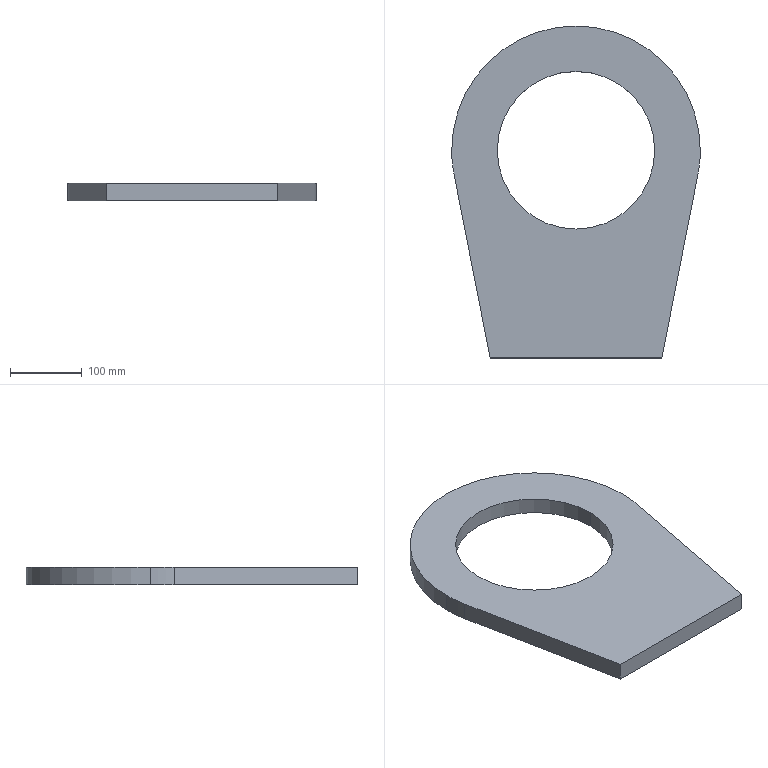Part | SolidWorks | features Extrusion 1, ICE 1 | 1 solid | 13 faces | box 347 x 463.5 x 25 mm | volume 2362679 mm3 | cylinder 7 | plane 6 | commonest cylinder face diameters 347 x3 220 x2 246 x2
STEP:
#1=CARTESIAN_POINT('',(-123.,290.,2.));
#2=VERTEX_POINT('',#1);
#3=CARTESIAN_POINT('',(123.,290.,2.));
#4=VERTEX_POINT('',#3);
#5=CARTESIAN_POINT('',(0.,290.,2.));
#6=DIRECTION('',(0.,0.,1.));
#7=DIRECTION('',(1.,0.,0.));
#8=AXIS2_PLACEMENT_3D('',#5,#6,#7);
#9=CIRCLE('',#8,123.);
#10=EDGE_CURVE('',#2,#4,#9,.T.);
#11=ORIENTED_EDGE('',*,*,#10,.T.);
#12=CARTESIAN_POINT('',(123.,290.,0.));
#13=VERTEX_POINT('',#12);
#14=CARTESIAN_POINT('',(123.,290.,2.));
#15=DIRECTION('',(0.,0.,-1.));
#16=VECTOR('',#15,1000.);
#17=LINE('',#14,#16);
#18=EDGE_CURVE('',#4,#13,#17,.T.);
#19=ORIENTED_EDGE('',*,*,#18,.T.);
#20=CARTESIAN_POINT('',(-123.,290.,0.));
#21=VERTEX_POINT('',#20);
#22=CARTESIAN_POINT('',(0.,290.,0.));
#23=DIRECTION('',(0.,0.,1.));
#24=DIRECTION('',(1.,0.,0.));
#25=AXIS2_PLACEMENT_3D('',#22,#23,#24);
#26=CIRCLE('',#25,123.);
#27=EDGE_CURVE('',#21,#13,#26,.T.);
#28=ORIENTED_EDGE('',*,*,#27,.F.);
#29=CARTESIAN_POINT('',(-123.,290.,2.));
#30=DIRECTION('',(0.,0.,-1.));
#31=VECTOR('',#30,1000.);
#32=LINE('',#29,#31);
#33=EDGE_CURVE('',#2,#21,#32,.T.);
#34=ORIENTED_EDGE('',*,*,#33,.F.);
#35=EDGE_LOOP('',(#11,#19,#28,#34));
#36=FACE_OUTER_BOUND('',#35,.T.);
#37=CARTESIAN_POINT('',(0.,290.,2.));
#38=DIRECTION('',(0.,0.,-1.));
#39=DIRECTION('',(-1.,0.,0.));
#40=AXIS2_PLACEMENT_3D('',#37,#38,#39);
#41=CYLINDRICAL_SURFACE('',#40,123.);
#42=ADVANCED_FACE('',(#36),#41,.F.);
#43=CARTESIAN_POINT('',(-110.,290.,25.));
#44=VERTEX_POINT('',#43);
#45=CARTESIAN_POINT('',(110.,290.,25.));
#46=VERTEX_POINT('',#45);
#47=CARTESIAN_POINT('',(0.,290.,25.));
#48=DIRECTION('',(0.,0.,1.));
#49=DIRECTION('',(1.,0.,0.));
#50=AXIS2_PLACEMENT_3D('',#47,#48,#49);
#51=CIRCLE('',#50,110.);
#52=EDGE_CURVE('',#44,#46,#51,.T.);
#53=ORIENTED_EDGE('',*,*,#52,.T.);
#54=CARTESIAN_POINT('',(110.,290.,2.));
#55=VERTEX_POINT('',#54);
#56=CARTESIAN_POINT('',(110.,290.,25.));
#57=DIRECTION('',(0.,0.,-1.));
#58=VECTOR('',#57,1000.);
#59=LINE('',#56,#58);
#60=EDGE_CURVE('',#46,#55,#59,.T.);
#61=ORIENTED_EDGE('',*,*,#60,.T.);
#62=CARTESIAN_POINT('',(-110.,290.,2.));
#63=VERTEX_POINT('',#62);
#64=CARTESIAN_POINT('',(0.,290.,2.));
#65=DIRECTION('',(0.,0.,1.));
#66=DIRECTION('',(1.,0.,0.));
#67=AXIS2_PLACEMENT_3D('',#64,#65,#66);
#68=CIRCLE('',#67,110.);
#69=EDGE_CURVE('',#63,#55,#68,.T.);
#70=ORIENTED_EDGE('',*,*,#69,.F.);
#71=CARTESIAN_POINT('',(-110.,290.,25.));
#72=DIRECTION('',(0.,0.,-1.));
#73=VECTOR('',#72,1000.);
#74=LINE('',#71,#73);
#75=EDGE_CURVE('',#44,#63,#74,.T.);
#76=ORIENTED_EDGE('',*,*,#75,.F.);
#77=EDGE_LOOP('',(#53,#61,#70,#76));
#78=FACE_OUTER_BOUND('',#77,.T.);
#79=CARTESIAN_POINT('',(0.,290.,25.));
#80=DIRECTION('',(0.,0.,-1.));
#81=DIRECTION('',(-1.,0.,0.));
#82=AXIS2_PLACEMENT_3D('',#79,#80,#81);
#83=CYLINDRICAL_SURFACE('',#82,110.);
#84=ADVANCED_FACE('',(#78),#83,.F.);
#85=CARTESIAN_POINT('',(173.5,290.,25.));
#86=VERTEX_POINT('',#85);
#87=CARTESIAN_POINT('',(-173.5,290.,25.));
#88=VERTEX_POINT('',#87);
#89=CARTESIAN_POINT('',(0.,290.,25.));
#90=DIRECTION('',(0.,0.,1.));
#91=DIRECTION('',(1.,0.,0.));
#92=AXIS2_PLACEMENT_3D('',#89,#90,#91);
#93=CIRCLE('',#92,173.5);
#94=EDGE_CURVE('',#86,#88,#93,.T.);
#95=ORIENTED_EDGE('',*,*,#94,.F.);
#96=CARTESIAN_POINT('',(173.5,290.,0.));
#97=VERTEX_POINT('',#96);
#98=CARTESIAN_POINT('',(173.5,290.,25.));
#99=DIRECTION('',(0.,0.,-1.));
#100=VECTOR('',#99,1000.);
#101=LINE('',#98,#100);
#102=EDGE_CURVE('',#86,#97,#101,.T.);
#103=ORIENTED_EDGE('',*,*,#102,.T.);
#104=CARTESIAN_POINT('',(-173.5,290.,0.));
#105=VERTEX_POINT('',#104);
#106=CARTESIAN_POINT('',(0.,290.,0.));
#107=DIRECTION('',(0.,0.,1.));
#108=DIRECTION('',(1.,0.,0.));
#109=AXIS2_PLACEMENT_3D('',#106,#107,#108);
#110=CIRCLE('',#109,173.5);
#111=EDGE_CURVE('',#97,#105,#110,.T.);
#112=ORIENTED_EDGE('',*,*,#111,.T.);
#113=CARTESIAN_POINT('',(-173.5,290.,25.));
#114=DIRECTION('',(0.,0.,-1.));
#115=VECTOR('',#114,1000.);
#116=LINE('',#113,#115);
#117=EDGE_CURVE('',#88,#105,#116,.T.);
#118=ORIENTED_EDGE('',*,*,#117,.F.);
#119=EDGE_LOOP('',(#95,#103,#112,#118));
#120=FACE_OUTER_BOUND('',#119,.T.);
#121=CARTESIAN_POINT('',(0.,290.,25.));
#122=DIRECTION('',(0.,0.,-1.));
#123=DIRECTION('',(-1.,0.,0.));
#124=AXIS2_PLACEMENT_3D('',#121,#122,#123);
#125=CYLINDRICAL_SURFACE('',#124,173.5);
#126=ADVANCED_FACE('',(#120),#125,.T.);
#127=CARTESIAN_POINT('',(-170.265,256.654,25.));
#128=VERTEX_POINT('',#127);
#129=CARTESIAN_POINT('',(0.,290.,25.));
#130=DIRECTION('',(0.,0.,1.));
#131=DIRECTION('',(1.,0.,0.));
#132=AXIS2_PLACEMENT_3D('',#129,#130,#131);
#133=CIRCLE('',#132,173.5);
#134=EDGE_CURVE('',#88,#128,#133,.T.);
#135=ORIENTED_EDGE('',*,*,#134,.F.);
#136=ORIENTED_EDGE('',*,*,#117,.T.);
#137=CARTESIAN_POINT('',(-170.265,256.654,0.));
#138=VERTEX_POINT('',#137);
#139=CARTESIAN_POINT('',(0.,290.,0.));
#140=DIRECTION('',(0.,0.,1.));
#141=DIRECTION('',(1.,0.,0.));
#142=AXIS2_PLACEMENT_3D('',#139,#140,#141);
#143=CIRCLE('',#142,173.5);
#144=EDGE_CURVE('',#105,#138,#143,.T.);
#145=ORIENTED_EDGE('',*,*,#144,.T.);
#146=CARTESIAN_POINT('',(-170.265,256.654,25.));
#147=DIRECTION('',(0.,0.,-1.));
#148=VECTOR('',#147,1000.);
#149=LINE('',#146,#148);
#150=EDGE_CURVE('',#128,#138,#149,.T.);
#151=ORIENTED_EDGE('',*,*,#150,.F.);
#152=EDGE_LOOP('',(#135,#136,#145,#151));
#153=FACE_OUTER_BOUND('',#152,.T.);
#154=CARTESIAN_POINT('',(0.,290.,25.));
#155=DIRECTION('',(0.,0.,-1.));
#156=DIRECTION('',(-1.,0.,0.));
#157=AXIS2_PLACEMENT_3D('',#154,#155,#156);
#158=CYLINDRICAL_SURFACE('',#157,173.5);
#159=ADVANCED_FACE('',(#153),#158,.T.);
#160=CARTESIAN_POINT('',(-120.,0.,0.));
#161=VERTEX_POINT('',#160);
#162=CARTESIAN_POINT('',(-120.,0.,0.));
#163=DIRECTION('',(0.1922,-0.9814,0.));
#164=VECTOR('',#163,1000.);
#165=LINE('',#162,#164);
#166=EDGE_CURVE('',#138,#161,#165,.T.);
#167=ORIENTED_EDGE('',*,*,#166,.F.);
#168=ORIENTED_EDGE('',*,*,#144,.F.);
#169=ORIENTED_EDGE('',*,*,#111,.F.);
#170=CARTESIAN_POINT('',(170.265,256.654,0.));
#171=VERTEX_POINT('',#170);
#172=CARTESIAN_POINT('',(0.,290.,0.));
#173=DIRECTION('',(0.,0.,1.));
#174=DIRECTION('',(1.,0.,0.));
#175=AXIS2_PLACEMENT_3D('',#172,#173,#174);
#176=CIRCLE('',#175,173.5);
#177=EDGE_CURVE('',#171,#97,#176,.T.);
#178=ORIENTED_EDGE('',*,*,#177,.F.);
#179=CARTESIAN_POINT('',(120.,0.,0.));
#180=VERTEX_POINT('',#179);
#181=CARTESIAN_POINT('',(120.,0.,0.));
#182=DIRECTION('',(0.1922,0.9814,0.));
#183=VECTOR('',#182,1000.);
#184=LINE('',#181,#183);
#185=EDGE_CURVE('',#180,#171,#184,.T.);
#186=ORIENTED_EDGE('',*,*,#185,.F.);
#187=CARTESIAN_POINT('',(-120.,0.,0.));
#188=DIRECTION('',(1.,0.,0.));
#189=VECTOR('',#188,1000.);
#190=LINE('',#187,#189);
#191=EDGE_CURVE('',#161,#180,#190,.T.);
#192=ORIENTED_EDGE('',*,*,#191,.F.);
#193=EDGE_LOOP('',(#167,#168,#169,#178,#186,#192));
#194=FACE_OUTER_BOUND('',#193,.T.);
#195=ORIENTED_EDGE('',*,*,#27,.T.);
#196=CARTESIAN_POINT('',(0.,290.,0.));
#197=DIRECTION('',(0.,0.,1.));
#198=DIRECTION('',(1.,0.,0.));
#199=AXIS2_PLACEMENT_3D('',#196,#197,#198);
#200=CIRCLE('',#199,123.);
#201=EDGE_CURVE('',#13,#21,#200,.T.);
#202=ORIENTED_EDGE('',*,*,#201,.T.);
#203=EDGE_LOOP('',(#195,#202));
#204=FACE_BOUND('',#203,.T.);
#205=CARTESIAN_POINT('',(0.,290.,0.));
#206=DIRECTION('',(0.,0.,1.));
#207=DIRECTION('',(1.,0.,0.));
#208=AXIS2_PLACEMENT_3D('',#205,#206,#207);
#209=PLANE('',#208);
#210=ADVANCED_FACE('',(#194,#204),#209,.F.);
#211=CARTESIAN_POINT('',(-120.,0.,25.));
#212=VERTEX_POINT('',#211);
#213=CARTESIAN_POINT('',(-120.,0.,25.));
#214=DIRECTION('',(0.1922,-0.9814,0.));
#215=VECTOR('',#214,1000.);
#216=LINE('',#213,#215);
#217=EDGE_CURVE('',#128,#212,#216,.T.);
#218=ORIENTED_EDGE('',*,*,#217,.T.);
#219=CARTESIAN_POINT('',(120.,0.,25.));
#220=VERTEX_POINT('',#219);
#221=CARTESIAN_POINT('',(-120.,0.,25.));
#222=DIRECTION('',(1.,0.,0.));
#223=VECTOR('',#222,1000.);
#224=LINE('',#221,#223);
#225=EDGE_CURVE('',#212,#220,#224,.T.);
#226=ORIENTED_EDGE('',*,*,#225,.T.);
#227=CARTESIAN_POINT('',(170.265,256.654,25.));
#228=VERTEX_POINT('',#227);
#229=CARTESIAN_POINT('',(120.,0.,25.));
#230=DIRECTION('',(0.1922,0.9814,0.));
#231=VECTOR('',#230,1000.);
#232=LINE('',#229,#231);
#233=EDGE_CURVE('',#220,#228,#232,.T.);
#234=ORIENTED_EDGE('',*,*,#233,.T.);
#235=CARTESIAN_POINT('',(0.,290.,25.));
#236=DIRECTION('',(0.,0.,1.));
#237=DIRECTION('',(1.,0.,0.));
#238=AXIS2_PLACEMENT_3D('',#235,#236,#237);
#239=CIRCLE('',#238,173.5);
#240=EDGE_CURVE('',#228,#86,#239,.T.);
#241=ORIENTED_EDGE('',*,*,#240,.T.);
#242=ORIENTED_EDGE('',*,*,#94,.T.);
#243=ORIENTED_EDGE('',*,*,#134,.T.);
#244=EDGE_LOOP('',(#218,#226,#234,#241,#242,#243));
#245=FACE_OUTER_BOUND('',#244,.T.);
#246=ORIENTED_EDGE('',*,*,#52,.F.);
#247=CARTESIAN_POINT('',(0.,290.,25.));
#248=DIRECTION('',(0.,0.,1.));
#249=DIRECTION('',(1.,0.,0.));
#250=AXIS2_PLACEMENT_3D('',#247,#248,#249);
#251=CIRCLE('',#250,110.);
#252=EDGE_CURVE('',#46,#44,#251,.T.);
#253=ORIENTED_EDGE('',*,*,#252,.F.);
#254=EDGE_LOOP('',(#246,#253));
#255=FACE_BOUND('',#254,.T.);
#256=CARTESIAN_POINT('',(0.,290.,25.));
#257=DIRECTION('',(0.,0.,1.));
#258=DIRECTION('',(1.,0.,0.));
#259=AXIS2_PLACEMENT_3D('',#256,#257,#258);
#260=PLANE('',#259);
#261=ADVANCED_FACE('',(#245,#255),#260,.T.);
#262=ORIENTED_EDGE('',*,*,#166,.T.);
#263=CARTESIAN_POINT('',(-120.,0.,25.));
#264=DIRECTION('',(0.,0.,-1.));
#265=VECTOR('',#264,1000.);
#266=LINE('',#263,#265);
#267=EDGE_CURVE('',#212,#161,#266,.T.);
#268=ORIENTED_EDGE('',*,*,#267,.F.);
#269=ORIENTED_EDGE('',*,*,#217,.F.);
#270=ORIENTED_EDGE('',*,*,#150,.T.);
#271=EDGE_LOOP('',(#262,#268,#269,#270));
#272=FACE_OUTER_BOUND('',#271,.T.);
#273=CARTESIAN_POINT('',(-120.,0.,25.));
#274=DIRECTION('',(0.9814,0.1922,0.));
#275=DIRECTION('',(-0.1922,0.9814,0.));
#276=AXIS2_PLACEMENT_3D('',#273,#274,#275);
#277=PLANE('',#276);
#278=ADVANCED_FACE('',(#272),#277,.F.);
#279=ORIENTED_EDGE('',*,*,#191,.T.);
#280=CARTESIAN_POINT('',(120.,0.,25.));
#281=DIRECTION('',(0.,0.,-1.));
#282=VECTOR('',#281,1000.);
#283=LINE('',#280,#282);
#284=EDGE_CURVE('',#220,#180,#283,.T.);
#285=ORIENTED_EDGE('',*,*,#284,.F.);
#286=ORIENTED_EDGE('',*,*,#225,.F.);
#287=ORIENTED_EDGE('',*,*,#267,.T.);
#288=EDGE_LOOP('',(#279,#285,#286,#287));
#289=FACE_OUTER_BOUND('',#288,.T.);
#290=CARTESIAN_POINT('',(-120.,0.,25.));
#291=DIRECTION('',(0.,1.,0.));
#292=DIRECTION('',(0.,0.,1.));
#293=AXIS2_PLACEMENT_3D('',#290,#291,#292);
#294=PLANE('',#293);
#295=ADVANCED_FACE('',(#289),#294,.F.);
#296=ORIENTED_EDGE('',*,*,#185,.T.);
#297=CARTESIAN_POINT('',(170.265,256.654,25.));
#298=DIRECTION('',(0.,0.,-1.));
#299=VECTOR('',#298,1000.);
#300=LINE('',#297,#299);
#301=EDGE_CURVE('',#228,#171,#300,.T.);
#302=ORIENTED_EDGE('',*,*,#301,.F.);
#303=ORIENTED_EDGE('',*,*,#233,.F.);
#304=ORIENTED_EDGE('',*,*,#284,.T.);
#305=EDGE_LOOP('',(#296,#302,#303,#304));
#306=FACE_OUTER_BOUND('',#305,.T.);
#307=CARTESIAN_POINT('',(120.,0.,25.));
#308=DIRECTION('',(-0.9814,0.1922,0.));
#309=DIRECTION('',(-0.1922,-0.9814,0.));
#310=AXIS2_PLACEMENT_3D('',#307,#308,#309);
#311=PLANE('',#310);
#312=ADVANCED_FACE('',(#306),#311,.F.);
#313=ORIENTED_EDGE('',*,*,#102,.F.);
#314=ORIENTED_EDGE('',*,*,#240,.F.);
#315=ORIENTED_EDGE('',*,*,#301,.T.);
#316=ORIENTED_EDGE('',*,*,#177,.T.);
#317=EDGE_LOOP('',(#313,#314,#315,#316));
#318=FACE_OUTER_BOUND('',#317,.T.);
#319=CARTESIAN_POINT('',(0.,290.,25.));
#320=DIRECTION('',(0.,0.,-1.));
#321=DIRECTION('',(-1.,0.,0.));
#322=AXIS2_PLACEMENT_3D('',#319,#320,#321);
#323=CYLINDRICAL_SURFACE('',#322,173.5);
#324=ADVANCED_FACE('',(#318),#323,.T.);
#325=ORIENTED_EDGE('',*,*,#60,.F.);
#326=ORIENTED_EDGE('',*,*,#252,.T.);
#327=ORIENTED_EDGE('',*,*,#75,.T.);
#328=CARTESIAN_POINT('',(0.,290.,2.));
#329=DIRECTION('',(0.,0.,1.));
#330=DIRECTION('',(1.,0.,0.));
#331=AXIS2_PLACEMENT_3D('',#328,#329,#330);
#332=CIRCLE('',#331,110.);
#333=EDGE_CURVE('',#55,#63,#332,.T.);
#334=ORIENTED_EDGE('',*,*,#333,.F.);
#335=EDGE_LOOP('',(#325,#326,#327,#334));
#336=FACE_OUTER_BOUND('',#335,.T.);
#337=CARTESIAN_POINT('',(0.,290.,25.));
#338=DIRECTION('',(0.,0.,-1.));
#339=DIRECTION('',(-1.,0.,0.));
#340=AXIS2_PLACEMENT_3D('',#337,#338,#339);
#341=CYLINDRICAL_SURFACE('',#340,110.);
#342=ADVANCED_FACE('',(#336),#341,.F.);
#343=ORIENTED_EDGE('',*,*,#10,.F.);
#344=CARTESIAN_POINT('',(0.,290.,2.));
#345=DIRECTION('',(0.,0.,1.));
#346=DIRECTION('',(1.,0.,0.));
#347=AXIS2_PLACEMENT_3D('',#344,#345,#346);
#348=CIRCLE('',#347,123.);
#349=EDGE_CURVE('',#4,#2,#348,.T.);
#350=ORIENTED_EDGE('',*,*,#349,.F.);
#351=EDGE_LOOP('',(#343,#350));
#352=FACE_OUTER_BOUND('',#351,.T.);
#353=ORIENTED_EDGE('',*,*,#69,.T.);
#354=ORIENTED_EDGE('',*,*,#333,.T.);
#355=EDGE_LOOP('',(#353,#354));
#356=FACE_BOUND('',#355,.T.);
#357=CARTESIAN_POINT('',(0.,290.,2.));
#358=DIRECTION('',(0.,0.,1.));
#359=DIRECTION('',(1.,0.,0.));
#360=AXIS2_PLACEMENT_3D('',#357,#358,#359);
#361=PLANE('',#360);
#362=ADVANCED_FACE('',(#352,#356),#361,.F.);
#363=ORIENTED_EDGE('',*,*,#18,.F.);
#364=ORIENTED_EDGE('',*,*,#349,.T.);
#365=ORIENTED_EDGE('',*,*,#33,.T.);
#366=ORIENTED_EDGE('',*,*,#201,.F.);
#367=EDGE_LOOP('',(#363,#364,#365,#366));
#368=FACE_OUTER_BOUND('',#367,.T.);
#369=CARTESIAN_POINT('',(0.,290.,2.));
#370=DIRECTION('',(0.,0.,-1.));
#371=DIRECTION('',(-1.,0.,0.));
#372=AXIS2_PLACEMENT_3D('',#369,#370,#371);
#373=CYLINDRICAL_SURFACE('',#372,123.);
#374=ADVANCED_FACE('',(#368),#373,.F.);
#375=CLOSED_SHELL('',(#42,#84,#126,#159,#210,#261,#278,#295,#312,#324,#342,#362,#374));
#376=MANIFOLD_SOLID_BREP('',#375);
#377=CARTESIAN_POINT('',(0.,0.,0.));
#378=DIRECTION('',(0.,0.,1.));
#379=DIRECTION('',(1.,0.,0.));
#380=AXIS2_PLACEMENT_3D('',#377,#378,#379);
#381=(LENGTH_UNIT()NAMED_UNIT(*)SI_UNIT(.MILLI.,.METRE.));
#382=UNCERTAINTY_MEASURE_WITH_UNIT(LENGTH_MEASURE(0.00001),#381,'','');
#383=(NAMED_UNIT(*)PLANE_ANGLE_UNIT()SI_UNIT($,.RADIAN.));
#384=(NAMED_UNIT(*)SI_UNIT($,.STERADIAN.)SOLID_ANGLE_UNIT());
#385=(GEOMETRIC_REPRESENTATION_CONTEXT(3)GLOBAL_UNCERTAINTY_ASSIGNED_CONTEXT((#382))GLOBAL_UNIT_ASSIGNED_CONTEXT((#381,#383,#384))REPRESENTATION_CONTEXT('',''));
#386=ADVANCED_BREP_SHAPE_REPRESENTATION('',(#376,#380),#385);